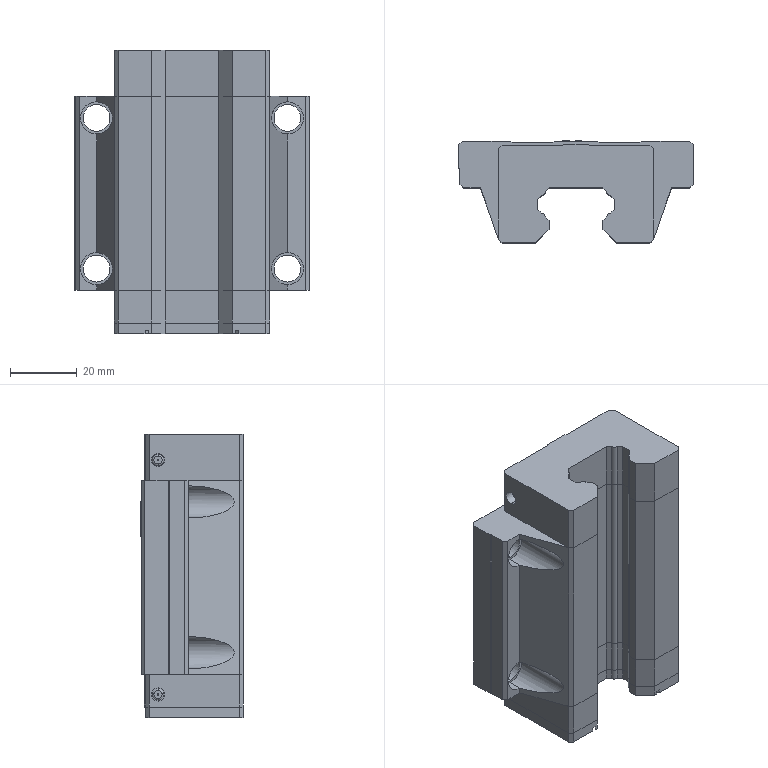Part | SolidWorks | features ICE 25, Extrusion 5, MirrorPattern 5, Fillet 4, MirrorSolid 4, Chamfer 3, RevCut 3, Dome 2, LPattern 2, Revolution 2, DeleteBody 1, LibraryFeature 1 | 4 solids | 730 faces | box 70 x 30.5 x 84.75 mm | volume 108873 mm3 | plane 491 | spline 160 | cylinder 67 | torus 10 | sphere 2 | commonest cylinder face diameters 2.258 x24 3.9 x12 9.6 x9 0.526 x8 8 x8 4.655 x4